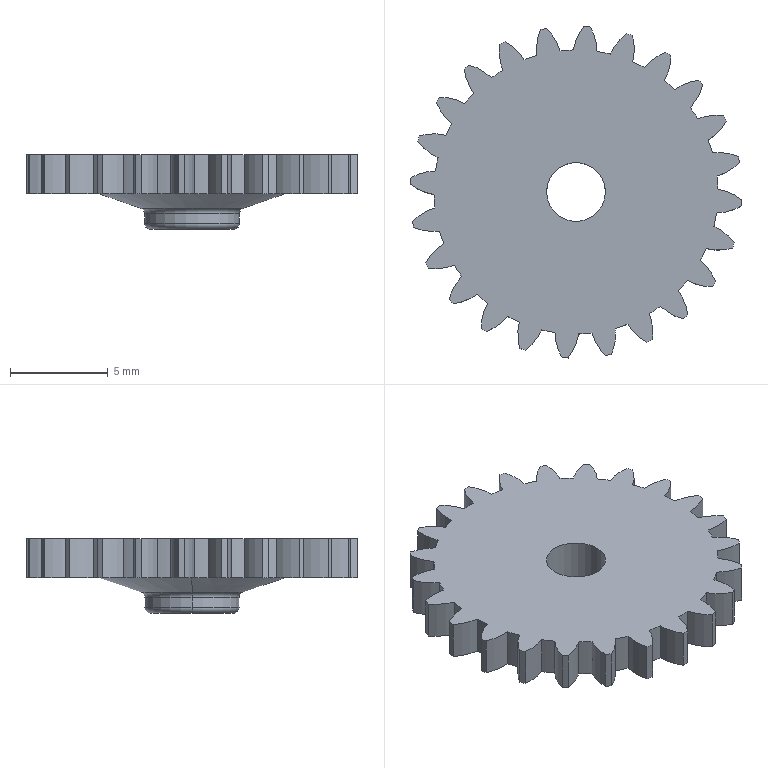Part | SolidWorks | features ICE 2, Blend 1, CirPattern 1, Cut 1, Extrusion 1, Fillet 1 | 1 solid | 113 faces | box 16.941 x 16.941 x 3.8 mm | volume 406.625 mm3 | cylinder 104 | torus 4 | plane 3 | cone 2 | commonest cylinder face diameters 5.301 x52 14.5 x24 16.96 x24 3 x2 4.841 x2